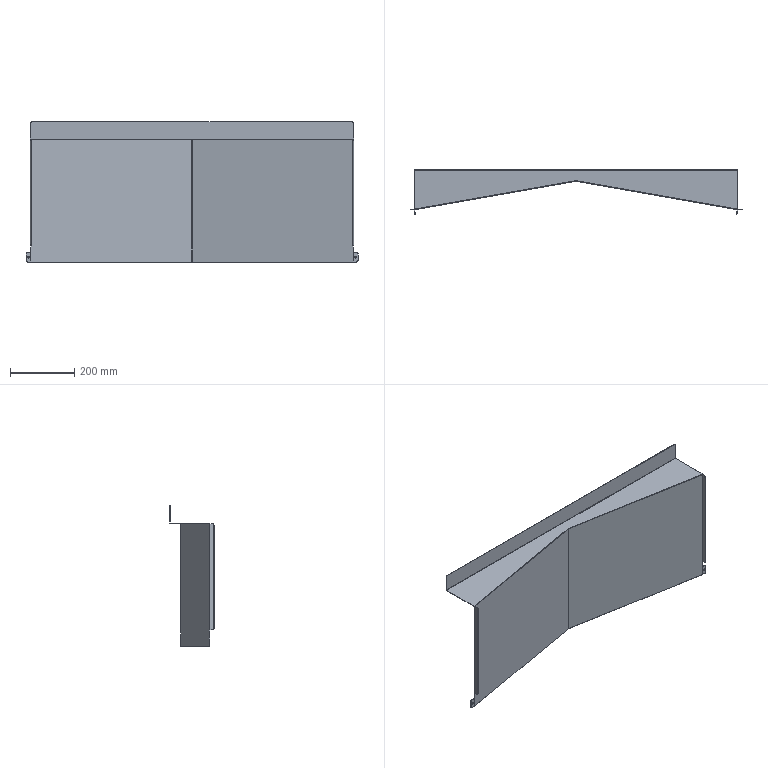Part | SolidWorks | features BaseBody 2 | 2 solids | 65 faces | box 1031 x 136.855 x 435 mm | volume 794680 mm3 | plane 35 | cylinder 30 | commonest cylinder face diameters 10 x10 1 x7 4 x7 5.5 x4 1.473 x1 4.473 x1